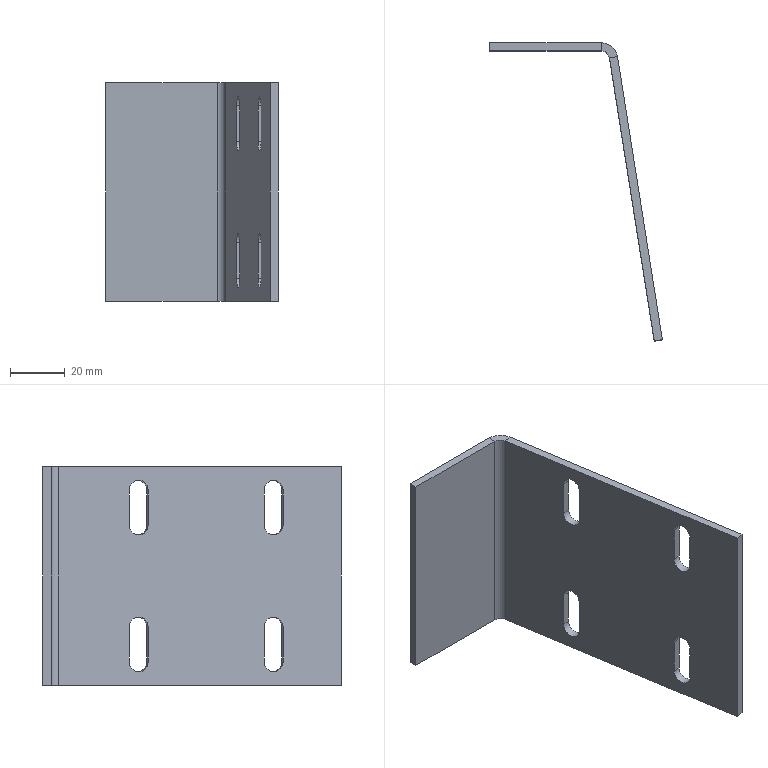Part | STEP file | 03-Stick plate 1 | 1 solid | 30 faces | box 63.208 x 109.115 x 80 mm | volume 34953 mm3 | plane 20 | cylinder 10 | commonest cylinder face diameters 7 x8 6 x1 12 x1